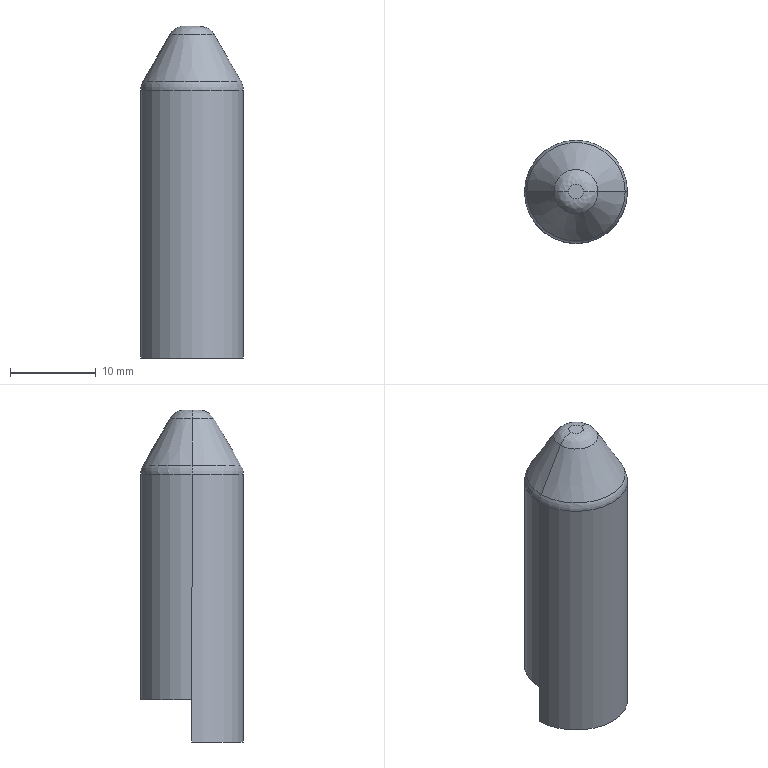Part | STEP file | 1 solid | 16 faces | box 12 x 12 x 38.7 mm | volume 3601 mm3 | plane 6 | cylinder 4 | other 2 | torus 2 | cone 2 | commonest cylinder face diameters 12 x2 5.2 x1 7.4 x1
STEP:
#1=CARTESIAN_POINT('',(0.,0.,0.));
#2=DIRECTION('',(0.,0.,1.));
#3=DIRECTION('',(1.,0.,0.));
#4=AXIS2_PLACEMENT_3D('',#1,#2,#3);
#5=CARTESIAN_POINT('',(6.,0.,-3.7));
#6=VERTEX_POINT('',#5);
#7=CARTESIAN_POINT('',(2.6,0.,-3.7));
#8=VERTEX_POINT('',#7);
#9=CARTESIAN_POINT('',(7.5,0.,-3.7));
#10=DIRECTION('',(-1.,0.,0.));
#11=VECTOR('',#10,1.);
#12=LINE('',#9,#11);
#13=CARTESIAN_POINT('',(7.5,0.,18.));
#14=DIRECTION('',(0.,-1.,0.));
#15=DIRECTION('',(-1.,0.,0.));
#16=AXIS2_PLACEMENT_3D('',#13,#14,#15);
#17=PLANE('',#16);
#18=CARTESIAN_POINT('',(0.,21.7));
#19=DIRECTION('',(1.,0.));
#20=VECTOR('',#19,1.);
#21=LINE('',#18,#20);
#22=(GEOMETRIC_REPRESENTATION_CONTEXT(2)PARAMETRIC_REPRESENTATION_CONTEXT()REPRESENTATION_CONTEXT('',''));
#23=DEFINITIONAL_REPRESENTATION('',(#21),#22);
#24=PCURVE('',#17,#23);
#25=CARTESIAN_POINT('',(0.,0.,-3.7));
#26=DIRECTION('',(0.,0.,1.));
#27=DIRECTION('',(1.,0.,0.));
#28=AXIS2_PLACEMENT_3D('',#25,#26,#27);
#29=PLANE('',#28);
#30=CARTESIAN_POINT('',(7.5,0.));
#31=DIRECTION('',(-1.,0.));
#32=VECTOR('',#31,1.);
#33=LINE('',#30,#32);
#34=(GEOMETRIC_REPRESENTATION_CONTEXT(2)PARAMETRIC_REPRESENTATION_CONTEXT()REPRESENTATION_CONTEXT('',''));
#35=DEFINITIONAL_REPRESENTATION('',(#33),#34);
#36=PCURVE('',#29,#35);
#37=SURFACE_CURVE('',#12,(#24,#36),.PCURVE_S1.);
#38=EDGE_CURVE('',#6,#8,#37,.T.);
#39=ORIENTED_EDGE('',*,*,#38,.T.);
#40=CARTESIAN_POINT('',(2.6,0.,-2.2));
#41=VERTEX_POINT('',#40);
#42=CARTESIAN_POINT('',(2.6,0.,-11.));
#43=DIRECTION('',(0.,0.,-1.));
#44=VECTOR('',#43,1.);
#45=LINE('',#42,#44);
#46=CARTESIAN_POINT('',(4.9,29.));
#47=DIRECTION('',(0.,1.));
#48=VECTOR('',#47,1.);
#49=LINE('',#46,#48);
#50=(GEOMETRIC_REPRESENTATION_CONTEXT(2)PARAMETRIC_REPRESENTATION_CONTEXT()REPRESENTATION_CONTEXT('',''));
#51=DEFINITIONAL_REPRESENTATION('',(#49),#50);
#52=PCURVE('',#17,#51);
#53=CARTESIAN_POINT('',(0.,0.,-11.));
#54=DIRECTION('',(0.,0.,-1.));
#55=DIRECTION('',(0.,1.,0.));
#56=AXIS2_PLACEMENT_3D('',#53,#54,#55);
#57=CYLINDRICAL_SURFACE('',#56,2.6);
#58=CARTESIAN_POINT('',(1.571,0.));
#59=DIRECTION('',(0.,1.));
#60=VECTOR('',#59,1.);
#61=LINE('',#58,#60);
#62=(GEOMETRIC_REPRESENTATION_CONTEXT(2)PARAMETRIC_REPRESENTATION_CONTEXT()REPRESENTATION_CONTEXT('',''));
#63=DEFINITIONAL_REPRESENTATION('',(#61),#62);
#64=PCURVE('',#57,#63);
#65=SURFACE_CURVE('',#45,(#52,#64),.PCURVE_S1.);
#66=EDGE_CURVE('',#41,#8,#65,.T.);
#67=ORIENTED_EDGE('',*,*,#66,.F.);
#68=CARTESIAN_POINT('',(3.7,0.,-2.2));
#69=VERTEX_POINT('',#68);
#70=CARTESIAN_POINT('',(0.,0.,-2.2));
#71=DIRECTION('',(-1.,0.,0.));
#72=VECTOR('',#71,1.);
#73=LINE('',#70,#72);
#74=CARTESIAN_POINT('',(7.5,20.2));
#75=DIRECTION('',(1.,0.));
#76=VECTOR('',#75,1.);
#77=LINE('',#74,#76);
#78=(GEOMETRIC_REPRESENTATION_CONTEXT(2)PARAMETRIC_REPRESENTATION_CONTEXT()REPRESENTATION_CONTEXT('',''));
#79=DEFINITIONAL_REPRESENTATION('',(#77),#78);
#80=PCURVE('',#17,#79);
#81=CARTESIAN_POINT('',(0.,3.7,-2.2));
#82=DIRECTION('',(0.,0.,-1.));
#83=DIRECTION('',(-1.,0.,0.));
#84=AXIS2_PLACEMENT_3D('',#81,#82,#83);
#85=PLANE('',#84);
#86=CARTESIAN_POINT('',(0.,-3.7));
#87=DIRECTION('',(1.,0.));
#88=VECTOR('',#87,1.);
#89=LINE('',#86,#88);
#90=(GEOMETRIC_REPRESENTATION_CONTEXT(2)PARAMETRIC_REPRESENTATION_CONTEXT()REPRESENTATION_CONTEXT('',''));
#91=DEFINITIONAL_REPRESENTATION('',(#89),#90);
#92=PCURVE('',#85,#91);
#93=SURFACE_CURVE('',#73,(#80,#92),.PCURVE_S1.);
#94=EDGE_CURVE('',#69,#41,#93,.T.);
#95=ORIENTED_EDGE('',*,*,#94,.F.);
#96=CARTESIAN_POINT('',(3.7,0.,1.2));
#97=VERTEX_POINT('',#96);
#98=CARTESIAN_POINT('',(3.7,0.,-11.));
#99=DIRECTION('',(0.,0.,-1.));
#100=VECTOR('',#99,1.);
#101=LINE('',#98,#100);
#102=CARTESIAN_POINT('',(3.8,29.));
#103=DIRECTION('',(0.,1.));
#104=VECTOR('',#103,1.);
#105=LINE('',#102,#104);
#106=(GEOMETRIC_REPRESENTATION_CONTEXT(2)PARAMETRIC_REPRESENTATION_CONTEXT()REPRESENTATION_CONTEXT('',''));
#107=DEFINITIONAL_REPRESENTATION('',(#105),#106);
#108=PCURVE('',#17,#107);
#109=CARTESIAN_POINT('',(0.,0.,-11.));
#110=DIRECTION('',(0.,0.,-1.));
#111=DIRECTION('',(0.,1.,0.));
#112=AXIS2_PLACEMENT_3D('',#109,#110,#111);
#113=CYLINDRICAL_SURFACE('',#112,3.7);
#114=CARTESIAN_POINT('',(1.571,0.));
#115=DIRECTION('',(0.,1.));
#116=VECTOR('',#115,1.);
#117=LINE('',#114,#116);
#118=(GEOMETRIC_REPRESENTATION_CONTEXT(2)PARAMETRIC_REPRESENTATION_CONTEXT()REPRESENTATION_CONTEXT('',''));
#119=DEFINITIONAL_REPRESENTATION('',(#117),#118);
#120=PCURVE('',#113,#119);
#121=SURFACE_CURVE('',#101,(#108,#120),.PCURVE_S1.);
#122=EDGE_CURVE('',#97,#69,#121,.T.);
#123=ORIENTED_EDGE('',*,*,#122,.F.);
#124=CARTESIAN_POINT('',(6.,0.,1.2));
#125=VERTEX_POINT('',#124);
#126=CARTESIAN_POINT('',(7.5,0.,1.2));
#127=DIRECTION('',(-1.,0.,0.));
#128=VECTOR('',#127,1.);
#129=LINE('',#126,#128);
#130=CARTESIAN_POINT('',(0.,16.8));
#131=DIRECTION('',(1.,0.));
#132=VECTOR('',#131,1.);
#133=LINE('',#130,#132);
#134=(GEOMETRIC_REPRESENTATION_CONTEXT(2)PARAMETRIC_REPRESENTATION_CONTEXT()REPRESENTATION_CONTEXT('',''));
#135=DEFINITIONAL_REPRESENTATION('',(#133),#134);
#136=PCURVE('',#17,#135);
#137=CARTESIAN_POINT('',(0.,0.,1.2));
#138=DIRECTION('',(0.,0.,1.));
#139=DIRECTION('',(0.,-1.,0.));
#140=AXIS2_PLACEMENT_3D('',#137,#138,#139);
#141=PLANE('',#140);
#142=CARTESIAN_POINT('',(0.,7.5));
#143=DIRECTION('',(0.,-1.));
#144=VECTOR('',#143,1.);
#145=LINE('',#142,#144);
#146=(GEOMETRIC_REPRESENTATION_CONTEXT(2)PARAMETRIC_REPRESENTATION_CONTEXT()REPRESENTATION_CONTEXT('',''));
#147=DEFINITIONAL_REPRESENTATION('',(#145),#146);
#148=PCURVE('',#141,#147);
#149=SURFACE_CURVE('',#129,(#136,#148),.PCURVE_S1.);
#150=EDGE_CURVE('',#125,#97,#149,.T.);
#151=ORIENTED_EDGE('',*,*,#150,.F.);
#152=CARTESIAN_POINT('',(6.,0.,35.));
#153=DIRECTION('',(0.,0.,1.));
#154=VECTOR('',#153,1.);
#155=LINE('',#152,#154);
#156=CARTESIAN_POINT('',(1.5,-17.));
#157=DIRECTION('',(0.,-1.));
#158=VECTOR('',#157,1.);
#159=LINE('',#156,#158);
#160=(GEOMETRIC_REPRESENTATION_CONTEXT(2)PARAMETRIC_REPRESENTATION_CONTEXT()REPRESENTATION_CONTEXT('',''));
#161=DEFINITIONAL_REPRESENTATION('',(#159),#160);
#162=PCURVE('',#17,#161);
#163=CARTESIAN_POINT('',(0.,0.,35.));
#164=DIRECTION('',(0.,0.,-1.));
#165=DIRECTION('',(-1.,0.,0.));
#166=AXIS2_PLACEMENT_3D('',#163,#164,#165);
#167=CYLINDRICAL_SURFACE('',#166,6.);
#168=CARTESIAN_POINT('',(3.142,0.));
#169=DIRECTION('',(0.,-1.));
#170=VECTOR('',#169,1.);
#171=LINE('',#168,#170);
#172=(GEOMETRIC_REPRESENTATION_CONTEXT(2)PARAMETRIC_REPRESENTATION_CONTEXT()REPRESENTATION_CONTEXT('',''));
#173=DEFINITIONAL_REPRESENTATION('',(#171),#172);
#174=PCURVE('',#167,#173);
#175=SURFACE_CURVE('',#155,(#162,#174),.PCURVE_S1.);
#176=EDGE_CURVE('',#6,#125,#175,.T.);
#177=ORIENTED_EDGE('',*,*,#176,.F.);
#178=EDGE_LOOP('',(#39,#67,#95,#123,#151,#177));
#179=FACE_BOUND('',#178,.T.);
#180=ADVANCED_FACE('',(#179),#17,.F.);
#181=CARTESIAN_POINT('',(-3.7,0.,1.2));
#182=VERTEX_POINT('',#181);
#183=CARTESIAN_POINT('',(-6.,0.,1.2));
#184=VERTEX_POINT('',#183);
#185=CARTESIAN_POINT('',(7.5,0.,1.2));
#186=DIRECTION('',(-1.,0.,0.));
#187=VECTOR('',#186,1.);
#188=LINE('',#185,#187);
#189=CARTESIAN_POINT('',(7.5,0.,18.));
#190=DIRECTION('',(0.,-1.,0.));
#191=DIRECTION('',(-1.,0.,0.));
#192=AXIS2_PLACEMENT_3D('',#189,#190,#191);
#193=PLANE('',#192);
#194=CARTESIAN_POINT('',(0.,16.8));
#195=DIRECTION('',(1.,0.));
#196=VECTOR('',#195,1.);
#197=LINE('',#194,#196);
#198=(GEOMETRIC_REPRESENTATION_CONTEXT(2)PARAMETRIC_REPRESENTATION_CONTEXT()REPRESENTATION_CONTEXT('',''));
#199=DEFINITIONAL_REPRESENTATION('',(#197),#198);
#200=PCURVE('',#193,#199);
#201=CARTESIAN_POINT('',(0.,7.5));
#202=DIRECTION('',(0.,-1.));
#203=VECTOR('',#202,1.);
#204=LINE('',#201,#203);
#205=(GEOMETRIC_REPRESENTATION_CONTEXT(2)PARAMETRIC_REPRESENTATION_CONTEXT()REPRESENTATION_CONTEXT('',''));
#206=DEFINITIONAL_REPRESENTATION('',(#204),#205);
#207=PCURVE('',#141,#206);
#208=SURFACE_CURVE('',#188,(#200,#207),.PCURVE_S1.);
#209=EDGE_CURVE('',#182,#184,#208,.T.);
#210=ORIENTED_EDGE('',*,*,#209,.F.);
#211=CARTESIAN_POINT('',(-3.7,0.,-2.2));
#212=VERTEX_POINT('',#211);
#213=CARTESIAN_POINT('',(-3.7,0.,-11.));
#214=DIRECTION('',(0.,0.,1.));
#215=VECTOR('',#214,1.);
#216=LINE('',#213,#215);
#217=CARTESIAN_POINT('',(11.2,29.));
#218=DIRECTION('',(0.,-1.));
#219=VECTOR('',#218,1.);
#220=LINE('',#217,#219);
#221=(GEOMETRIC_REPRESENTATION_CONTEXT(2)PARAMETRIC_REPRESENTATION_CONTEXT()REPRESENTATION_CONTEXT('',''));
#222=DEFINITIONAL_REPRESENTATION('',(#220),#221);
#223=PCURVE('',#193,#222);
#224=CARTESIAN_POINT('',(4.712,0.));
#225=DIRECTION('',(0.,-1.));
#226=VECTOR('',#225,1.);
#227=LINE('',#224,#226);
#228=(GEOMETRIC_REPRESENTATION_CONTEXT(2)PARAMETRIC_REPRESENTATION_CONTEXT()REPRESENTATION_CONTEXT('',''));
#229=DEFINITIONAL_REPRESENTATION('',(#227),#228);
#230=PCURVE('',#113,#229);
#231=SURFACE_CURVE('',#216,(#223,#230),.PCURVE_S1.);
#232=EDGE_CURVE('',#212,#182,#231,.T.);
#233=ORIENTED_EDGE('',*,*,#232,.F.);
#234=CARTESIAN_POINT('',(-2.6,0.,-2.2));
#235=VERTEX_POINT('',#234);
#236=CARTESIAN_POINT('',(0.,0.,-2.2));
#237=DIRECTION('',(-1.,0.,0.));
#238=VECTOR('',#237,1.);
#239=LINE('',#236,#238);
#240=CARTESIAN_POINT('',(7.5,20.2));
#241=DIRECTION('',(1.,0.));
#242=VECTOR('',#241,1.);
#243=LINE('',#240,#242);
#244=(GEOMETRIC_REPRESENTATION_CONTEXT(2)PARAMETRIC_REPRESENTATION_CONTEXT()REPRESENTATION_CONTEXT('',''));
#245=DEFINITIONAL_REPRESENTATION('',(#243),#244);
#246=PCURVE('',#193,#245);
#247=CARTESIAN_POINT('',(0.,-3.7));
#248=DIRECTION('',(1.,0.));
#249=VECTOR('',#248,1.);
#250=LINE('',#247,#249);
#251=(GEOMETRIC_REPRESENTATION_CONTEXT(2)PARAMETRIC_REPRESENTATION_CONTEXT()REPRESENTATION_CONTEXT('',''));
#252=DEFINITIONAL_REPRESENTATION('',(#250),#251);
#253=PCURVE('',#85,#252);
#254=SURFACE_CURVE('',#239,(#246,#253),.PCURVE_S1.);
#255=EDGE_CURVE('',#235,#212,#254,.T.);
#256=ORIENTED_EDGE('',*,*,#255,.F.);
#257=CARTESIAN_POINT('',(-2.6,0.,-3.7));
#258=VERTEX_POINT('',#257);
#259=CARTESIAN_POINT('',(-2.6,0.,-3.7));
#260=DIRECTION('',(0.,0.,1.));
#261=VECTOR('',#260,1.);
#262=LINE('',#259,#261);
#263=CARTESIAN_POINT('',(10.1,21.7));
#264=DIRECTION('',(0.,-1.));
#265=VECTOR('',#264,1.);
#266=LINE('',#263,#265);
#267=(GEOMETRIC_REPRESENTATION_CONTEXT(2)PARAMETRIC_REPRESENTATION_CONTEXT()REPRESENTATION_CONTEXT('',''));
#268=DEFINITIONAL_REPRESENTATION('',(#266),#267);
#269=PCURVE('',#193,#268);
#270=CARTESIAN_POINT('',(4.712,-7.3));
#271=DIRECTION('',(0.,-1.));
#272=VECTOR('',#271,1.);
#273=LINE('',#270,#272);
#274=(GEOMETRIC_REPRESENTATION_CONTEXT(2)PARAMETRIC_REPRESENTATION_CONTEXT()REPRESENTATION_CONTEXT('',''));
#275=DEFINITIONAL_REPRESENTATION('',(#273),#274);
#276=PCURVE('',#57,#275);
#277=SURFACE_CURVE('',#262,(#269,#276),.PCURVE_S1.);
#278=EDGE_CURVE('',#258,#235,#277,.T.);
#279=ORIENTED_EDGE('',*,*,#278,.F.);
#280=CARTESIAN_POINT('',(-6.,0.,-3.7));
#281=VERTEX_POINT('',#280);
#282=CARTESIAN_POINT('',(7.5,0.,-3.7));
#283=DIRECTION('',(-1.,0.,0.));
#284=VECTOR('',#283,1.);
#285=LINE('',#282,#284);
#286=CARTESIAN_POINT('',(0.,21.7));
#287=DIRECTION('',(1.,0.));
#288=VECTOR('',#287,1.);
#289=LINE('',#286,#288);
#290=(GEOMETRIC_REPRESENTATION_CONTEXT(2)PARAMETRIC_REPRESENTATION_CONTEXT()REPRESENTATION_CONTEXT('',''));
#291=DEFINITIONAL_REPRESENTATION('',(#289),#290);
#292=PCURVE('',#193,#291);
#293=CARTESIAN_POINT('',(7.5,0.));
#294=DIRECTION('',(-1.,0.));
#295=VECTOR('',#294,1.);
#296=LINE('',#293,#295);
#297=(GEOMETRIC_REPRESENTATION_CONTEXT(2)PARAMETRIC_REPRESENTATION_CONTEXT()REPRESENTATION_CONTEXT('',''));
#298=DEFINITIONAL_REPRESENTATION('',(#296),#297);
#299=PCURVE('',#29,#298);
#300=SURFACE_CURVE('',#285,(#292,#299),.PCURVE_S1.);
#301=EDGE_CURVE('',#258,#281,#300,.T.);
#302=ORIENTED_EDGE('',*,*,#301,.T.);
#303=CARTESIAN_POINT('',(-6.,0.,35.));
#304=DIRECTION('',(0.,0.,-1.));
#305=VECTOR('',#304,1.);
#306=LINE('',#303,#305);
#307=CARTESIAN_POINT('',(13.5,-17.));
#308=DIRECTION('',(0.,1.));
#309=VECTOR('',#308,1.);
#310=LINE('',#307,#309);
#311=(GEOMETRIC_REPRESENTATION_CONTEXT(2)PARAMETRIC_REPRESENTATION_CONTEXT()REPRESENTATION_CONTEXT('',''));
#312=DEFINITIONAL_REPRESENTATION('',(#310),#311);
#313=PCURVE('',#193,#312);
#314=CARTESIAN_POINT('',(6.283,0.));
#315=DIRECTION('',(0.,1.));
#316=VECTOR('',#315,1.);
#317=LINE('',#314,#316);
#318=(GEOMETRIC_REPRESENTATION_CONTEXT(2)PARAMETRIC_REPRESENTATION_CONTEXT()REPRESENTATION_CONTEXT('',''));
#319=DEFINITIONAL_REPRESENTATION('',(#317),#318);
#320=PCURVE('',#167,#319);
#321=SURFACE_CURVE('',#306,(#313,#320),.PCURVE_S1.);
#322=EDGE_CURVE('',#184,#281,#321,.T.);
#323=ORIENTED_EDGE('',*,*,#322,.F.);
#324=EDGE_LOOP('',(#210,#233,#256,#279,#302,#323));
#325=FACE_BOUND('',#324,.T.);
#326=ADVANCED_FACE('',(#325),#193,.F.);
#327=CARTESIAN_POINT('',(0.,0.,-2.2));
#328=DIRECTION('',(0.,0.,-1.));
#329=DIRECTION('',(0.,1.,0.));
#330=AXIS2_PLACEMENT_3D('',#327,#328,#329);
#331=CIRCLE('',#330,3.7);
#332=CARTESIAN_POINT('',(0.,-3.7));
#333=DIRECTION('',(0.,1.));
#334=AXIS2_PLACEMENT_2D('',#332,#333);
#335=CIRCLE('',#334,3.7);
#336=(GEOMETRIC_REPRESENTATION_CONTEXT(2)PARAMETRIC_REPRESENTATION_CONTEXT()REPRESENTATION_CONTEXT('',''));
#337=DEFINITIONAL_REPRESENTATION('',(#335),#336);
#338=PCURVE('',#85,#337);
#339=CARTESIAN_POINT('',(0.,-8.8));
#340=DIRECTION('',(1.,0.));
#341=VECTOR('',#340,1.);
#342=LINE('',#339,#341);
#343=(GEOMETRIC_REPRESENTATION_CONTEXT(2)PARAMETRIC_REPRESENTATION_CONTEXT()REPRESENTATION_CONTEXT('',''));
#344=DEFINITIONAL_REPRESENTATION('',(#342),#343);
#345=PCURVE('',#113,#344);
#346=SURFACE_CURVE('',#331,(#338,#345),.PCURVE_S1.);
#347=EDGE_CURVE('',#69,#212,#346,.T.);
#348=ORIENTED_EDGE('',*,*,#347,.F.);
#349=ORIENTED_EDGE('',*,*,#94,.T.);
#350=CARTESIAN_POINT('',(0.,0.,-2.2));
#351=DIRECTION('',(0.,0.,-1.));
#352=DIRECTION('',(0.,1.,0.));
#353=AXIS2_PLACEMENT_3D('',#350,#351,#352);
#354=CIRCLE('',#353,2.6);
#355=CARTESIAN_POINT('',(0.,-3.7));
#356=DIRECTION('',(0.,1.));
#357=AXIS2_PLACEMENT_2D('',#355,#356);
#358=CIRCLE('',#357,2.6);
#359=(GEOMETRIC_REPRESENTATION_CONTEXT(2)PARAMETRIC_REPRESENTATION_CONTEXT()REPRESENTATION_CONTEXT('',''));
#360=DEFINITIONAL_REPRESENTATION('',(#358),#359);
#361=PCURVE('',#85,#360);
#362=CARTESIAN_POINT('',(0.,-8.8));
#363=DIRECTION('',(1.,0.));
#364=VECTOR('',#363,1.);
#365=LINE('',#362,#364);
#366=(GEOMETRIC_REPRESENTATION_CONTEXT(2)PARAMETRIC_REPRESENTATION_CONTEXT()REPRESENTATION_CONTEXT('',''));
#367=DEFINITIONAL_REPRESENTATION('',(#365),#366);
#368=PCURVE('',#57,#367);
#369=SURFACE_CURVE('',#354,(#361,#368),.PCURVE_S1.);
#370=EDGE_CURVE('',#41,#235,#369,.T.);
#371=ORIENTED_EDGE('',*,*,#370,.T.);
#372=ORIENTED_EDGE('',*,*,#255,.T.);
#373=EDGE_LOOP('',(#348,#349,#371,#372));
#374=FACE_BOUND('',#373,.T.);
#375=ADVANCED_FACE('',(#374),#85,.F.);
#376=ORIENTED_EDGE('',*,*,#122,.F.);
#377=CARTESIAN_POINT('',(0.,0.,1.2));
#378=DIRECTION('',(0.,0.,-1.));
#379=DIRECTION('',(0.,-1.,0.));
#380=AXIS2_PLACEMENT_3D('',#377,#378,#379);
#381=CIRCLE('',#380,3.7);
#382=CARTESIAN_POINT('',(-3.142,-12.2));
#383=DIRECTION('',(1.,0.));
#384=VECTOR('',#383,1.);
#385=LINE('',#382,#384);
#386=(GEOMETRIC_REPRESENTATION_CONTEXT(2)PARAMETRIC_REPRESENTATION_CONTEXT()REPRESENTATION_CONTEXT('',''));
#387=DEFINITIONAL_REPRESENTATION('',(#385),#386);
#388=PCURVE('',#113,#387);
#389=CARTESIAN_POINT('',(3.7,0.));
#390=CARTESIAN_POINT('',(3.7,-6.409));
#391=CARTESIAN_POINT('',(-1.85,-3.204));
#392=CARTESIAN_POINT('',(-7.4,0.));
#393=CARTESIAN_POINT('',(-1.85,3.204));
#394=CARTESIAN_POINT('',(3.7,6.409));
#395=CARTESIAN_POINT('',(3.7,0.));
#396=(BOUNDED_CURVE()B_SPLINE_CURVE(2,(#389,#390,#391,#392,#393,#394,#395),.UNSPECIFIED.,.T.,.F.)B_SPLINE_CURVE_WITH_KNOTS((1,2,2,2,2,1),(-2.094,0.,2.094,4.189,6.283,8.378),.UNSPECIFIED.)CURVE()GEOMETRIC_REPRESENTATION_ITEM()RATIONAL_B_SPLINE_CURVE((1.,0.5,1.,0.5,1.,0.5,1.))REPRESENTATION_ITEM(''));
#397=(GEOMETRIC_REPRESENTATION_CONTEXT(2)PARAMETRIC_REPRESENTATION_CONTEXT()REPRESENTATION_CONTEXT('',''));
#398=DEFINITIONAL_REPRESENTATION('',(#396),#397);
#399=PCURVE('',#141,#398);
#400=SURFACE_CURVE('',#381,(#388,#399),.PCURVE_S1.);
#401=EDGE_CURVE('',#97,#182,#400,.T.);
#402=ORIENTED_EDGE('',*,*,#401,.T.);
#403=ORIENTED_EDGE('',*,*,#232,.F.);
#404=ORIENTED_EDGE('',*,*,#347,.F.);
#405=EDGE_LOOP('',(#376,#402,#403,#404));
#406=FACE_BOUND('',#405,.F.);
#407=ADVANCED_FACE('',(#406),#113,.F.);
#408=ORIENTED_EDGE('',*,*,#401,.T.);
#409=ORIENTED_EDGE('',*,*,#209,.T.);
#410=CARTESIAN_POINT('',(0.,0.,1.2));
#411=DIRECTION('',(0.,0.,1.));
#412=DIRECTION('',(0.,-1.,0.));
#413=AXIS2_PLACEMENT_3D('',#410,#411,#412);
#414=CIRCLE('',#413,6.);
#415=CARTESIAN_POINT('',(0.,0.));
#416=DIRECTION('',(1.,0.));
#417=AXIS2_PLACEMENT_2D('',#415,#416);
#418=CIRCLE('',#417,6.);
#419=(GEOMETRIC_REPRESENTATION_CONTEXT(2)PARAMETRIC_REPRESENTATION_CONTEXT()REPRESENTATION_CONTEXT('',''));
#420=DEFINITIONAL_REPRESENTATION('',(#418),#419);
#421=PCURVE('',#141,#420);
#422=CARTESIAN_POINT('',(0.,0.,35.));
#423=DIRECTION('',(0.,0.,-1.));
#424=DIRECTION('',(-1.,0.,0.));
#425=AXIS2_PLACEMENT_3D('',#422,#423,#424);
#426=CYLINDRICAL_SURFACE('',#425,6.);
#427=CARTESIAN_POINT('',(4.712,33.8));
#428=DIRECTION('',(-1.,0.));
#429=VECTOR('',#428,1.);
#430=LINE('',#427,#429);
#431=(GEOMETRIC_REPRESENTATION_CONTEXT(2)PARAMETRIC_REPRESENTATION_CONTEXT()REPRESENTATION_CONTEXT('',''));
#432=DEFINITIONAL_REPRESENTATION('',(#430),#431);
#433=PCURVE('',#426,#432);
#434=SURFACE_CURVE('',#414,(#421,#433),.PCURVE_S1.);
#435=EDGE_CURVE('',#125,#184,#434,.T.);
#436=ORIENTED_EDGE('',*,*,#435,.F.);
#437=ORIENTED_EDGE('',*,*,#150,.T.);
#438=EDGE_LOOP('',(#408,#409,#436,#437));
#439=FACE_BOUND('',#438,.T.);
#440=ADVANCED_FACE('',(#439),#141,.F.);
#441=ORIENTED_EDGE('',*,*,#66,.F.);
#442=ORIENTED_EDGE('',*,*,#370,.T.);
#443=ORIENTED_EDGE('',*,*,#278,.F.);
#444=CARTESIAN_POINT('',(0.,0.,-3.7));
#445=DIRECTION('',(0.,0.,1.));
#446=DIRECTION('',(1.,0.,0.));
#447=AXIS2_PLACEMENT_3D('',#444,#445,#446);
#448=CIRCLE('',#447,2.6);
#449=CARTESIAN_POINT('',(7.854,-7.3));
#450=DIRECTION('',(-1.,0.));
#451=VECTOR('',#450,1.);
#452=LINE('',#449,#451);
#453=(GEOMETRIC_REPRESENTATION_CONTEXT(2)PARAMETRIC_REPRESENTATION_CONTEXT()REPRESENTATION_CONTEXT('',''));
#454=DEFINITIONAL_REPRESENTATION('',(#452),#453);
#455=PCURVE('',#57,#454);
#456=CARTESIAN_POINT('',(0.,0.));
#457=DIRECTION('',(1.,0.));
#458=AXIS2_PLACEMENT_2D('',#456,#457);
#459=CIRCLE('',#458,2.6);
#460=(GEOMETRIC_REPRESENTATION_CONTEXT(2)PARAMETRIC_REPRESENTATION_CONTEXT()REPRESENTATION_CONTEXT('',''));
#461=DEFINITIONAL_REPRESENTATION('',(#459),#460);
#462=PCURVE('',#29,#461);
#463=SURFACE_CURVE('',#448,(#455,#462),.PCURVE_S1.);
#464=EDGE_CURVE('',#258,#8,#463,.T.);
#465=ORIENTED_EDGE('',*,*,#464,.T.);
#466=EDGE_LOOP('',(#441,#442,#443,#465));
#467=FACE_BOUND('',#466,.F.);
#468=ADVANCED_FACE('',(#467),#57,.F.);
#469=CARTESIAN_POINT('',(-2.577,0.,34.));
#470=VERTEX_POINT('',#469);
#471=CARTESIAN_POINT('',(-0.8453,0.,35.));
#472=VERTEX_POINT('',#471);
#473=CARTESIAN_POINT('',(-0.8453,0.,33.));
#474=DIRECTION('',(0.,1.,0.));
#475=DIRECTION('',(-1.,0.,0.));
#476=AXIS2_PLACEMENT_3D('',#473,#474,#475);
#477=CIRCLE('',#476,2.);
#478=CARTESIAN_POINT('',(2.577,0.,34.));
#479=CARTESIAN_POINT('',(2.403,0.,34.302));
#480=CARTESIAN_POINT('',(2.165,0.,34.568));
#481=CARTESIAN_POINT('',(1.873,0.,34.781));
#482=CARTESIAN_POINT('',(1.543,0.,34.927));
#483=CARTESIAN_POINT('',(1.194,0.,35.));
#484=CARTESIAN_POINT('',(0.8453,0.,35.));
#485=B_SPLINE_CURVE_WITH_KNOTS('',6,(#478,#479,#480,#481,#482,#483,#484),.UNSPECIFIED.,.F.,.F.,(7,7),(0.5236,1.571),.PIECEWISE_BEZIER_KNOTS.);
#486=CARTESIAN_POINT('',(0.,0.,33.));
#487=DIRECTION('',(0.,0.,1.));
#488=AXIS1_PLACEMENT('',#486,#487);
#489=SURFACE_OF_REVOLUTION('',#485,#488);
#490=CARTESIAN_POINT('',(3.142,0.));
#491=DIRECTION('',(0.,1.));
#492=VECTOR('',#491,1.);
#493=LINE('',#490,#492);
#494=(GEOMETRIC_REPRESENTATION_CONTEXT(2)PARAMETRIC_REPRESENTATION_CONTEXT()REPRESENTATION_CONTEXT('',''));
#495=DEFINITIONAL_REPRESENTATION('',(#493),#494);
#496=PCURVE('',#489,#495);
#497=CARTESIAN_POINT('',(2.577,0.,34.));
#498=CARTESIAN_POINT('',(2.403,0.,34.302));
#499=CARTESIAN_POINT('',(2.165,0.,34.568));
#500=CARTESIAN_POINT('',(1.873,0.,34.781));
#501=CARTESIAN_POINT('',(1.543,0.,34.927));
#502=CARTESIAN_POINT('',(1.194,0.,35.));
#503=CARTESIAN_POINT('',(0.8453,0.,35.));
#504=B_SPLINE_CURVE_WITH_KNOTS('',6,(#497,#498,#499,#500,#501,#502,#503),.UNSPECIFIED.,.F.,.F.,(7,7),(0.5236,1.571),.PIECEWISE_BEZIER_KNOTS.);
#505=CARTESIAN_POINT('',(0.,0.,33.));
#506=DIRECTION('',(0.,0.,1.));
#507=AXIS1_PLACEMENT('',#505,#506);
#508=SURFACE_OF_REVOLUTION('',#504,#507);
#509=CARTESIAN_POINT('',(3.142,0.));
#510=DIRECTION('',(0.,1.));
#511=VECTOR('',#510,1.);
#512=LINE('',#509,#511);
#513=(GEOMETRIC_REPRESENTATION_CONTEXT(2)PARAMETRIC_REPRESENTATION_CONTEXT()REPRESENTATION_CONTEXT('',''));
#514=DEFINITIONAL_REPRESENTATION('',(#512),#513);
#515=PCURVE('',#508,#514);
#516=SURFACE_CURVE('',#477,(#496,#515),.PCURVE_S1.);
#517=EDGE_CURVE('',#470,#472,#516,.T.);
#518=ORIENTED_EDGE('',*,*,#517,.F.);
#519=CARTESIAN_POINT('',(2.577,0.,34.));
#520=VERTEX_POINT('',#519);
#521=CARTESIAN_POINT('',(0.,0.,34.));
#522=DIRECTION('',(0.,0.,-1.));
#523=DIRECTION('',(1.,0.,0.));
#524=AXIS2_PLACEMENT_3D('',#521,#522,#523);
#525=CIRCLE('',#524,2.577);
#526=CARTESIAN_POINT('',(6.283,0.5236));
#527=DIRECTION('',(-1.,0.));
#528=VECTOR('',#527,1.);
#529=LINE('',#526,#528);
#530=(GEOMETRIC_REPRESENTATION_CONTEXT(2)PARAMETRIC_REPRESENTATION_CONTEXT()REPRESENTATION_CONTEXT('',''));
#531=DEFINITIONAL_REPRESENTATION('',(#529),#530);
#532=PCURVE('',#489,#531);
#533=CARTESIAN_POINT('',(0.,0.,35.));
#534=DIRECTION('',(0.,0.,-1.));
#535=DIRECTION('',(-1.,0.,0.));
#536=AXIS2_PLACEMENT_3D('',#533,#534,#535);
#537=CONICAL_SURFACE('',#536,2.,0.5236);
#538=CARTESIAN_POINT('',(3.142,1.));
#539=DIRECTION('',(1.,0.));
#540=VECTOR('',#539,1.);
#541=LINE('',#538,#540);
#542=(GEOMETRIC_REPRESENTATION_CONTEXT(2)PARAMETRIC_REPRESENTATION_CONTEXT()REPRESENTATION_CONTEXT('',''));
#543=DEFINITIONAL_REPRESENTATION('',(#541),#542);
#544=PCURVE('',#537,#543);
#545=SURFACE_CURVE('',#525,(#532,#544),.PCURVE_S1.);
#546=EDGE_CURVE('',#520,#470,#545,.T.);
#547=ORIENTED_EDGE('',*,*,#546,.F.);
#548=CARTESIAN_POINT('',(0.8453,0.,35.));
#549=VERTEX_POINT('',#548);
#550=CARTESIAN_POINT('',(0.8453,0.,33.));
#551=DIRECTION('',(0.,-1.,0.));
#552=DIRECTION('',(0.,0.,-1.));
#553=AXIS2_PLACEMENT_3D('',#550,#551,#552);
#554=CIRCLE('',#553,2.);
#555=CARTESIAN_POINT('',(6.283,-1.571));
#556=DIRECTION('',(0.,1.));
#557=VECTOR('',#556,1.);
#558=LINE('',#555,#557);
#559=(GEOMETRIC_REPRESENTATION_CONTEXT(2)PARAMETRIC_REPRESENTATION_CONTEXT()REPRESENTATION_CONTEXT('',''));
#560=DEFINITIONAL_REPRESENTATION('',(#558),#559);
#561=PCURVE('',#489,#560);
#562=CARTESIAN_POINT('',(0.,-1.571));
#563=DIRECTION('',(0.,1.));
#564=VECTOR('',#563,1.);
#565=LINE('',#562,#564);
#566=(GEOMETRIC_REPRESENTATION_CONTEXT(2)PARAMETRIC_REPRESENTATION_CONTEXT()REPRESENTATION_CONTEXT('',''));
#567=DEFINITIONAL_REPRESENTATION('',(#565),#566);
#568=PCURVE('',#508,#567);
#569=SURFACE_CURVE('',#554,(#561,#568),.PCURVE_S1.);
#570=EDGE_CURVE('',#520,#549,#569,.T.);
#571=ORIENTED_EDGE('',*,*,#570,.T.);
#572=CARTESIAN_POINT('',(0.,0.,35.));
#573=DIRECTION('',(0.,0.,1.));
#574=DIRECTION('',(1.,0.,0.));
#575=AXIS2_PLACEMENT_3D('',#572,#573,#574);
#576=CIRCLE('',#575,0.8453);
#577=CARTESIAN_POINT('',(0.,1.571));
#578=DIRECTION('',(1.,0.));
#579=VECTOR('',#578,1.);
#580=LINE('',#577,#579);
#581=(GEOMETRIC_REPRESENTATION_CONTEXT(2)PARAMETRIC_REPRESENTATION_CONTEXT()REPRESENTATION_CONTEXT('',''));
#582=DEFINITIONAL_REPRESENTATION('',(#580),#581);
#583=PCURVE('',#489,#582);
#584=CARTESIAN_POINT('',(0.,0.,35.));
#585=DIRECTION('',(0.,0.,1.));
#586=DIRECTION('',(1.,0.,0.));
#587=AXIS2_PLACEMENT_3D('',#584,#585,#586);
#588=PLANE('',#587);
#589=CARTESIAN_POINT('',(0.,0.));
#590=DIRECTION('',(1.,0.));
#591=AXIS2_PLACEMENT_2D('',#589,#590);
#592=CIRCLE('',#591,0.8453);
#593=(GEOMETRIC_REPRESENTATION_CONTEXT(2)PARAMETRIC_REPRESENTATION_CONTEXT()REPRESENTATION_CONTEXT('',''));
#594=DEFINITIONAL_REPRESENTATION('',(#592),#593);
#595=PCURVE('',#588,#594);
#596=SURFACE_CURVE('',#576,(#583,#595),.PCURVE_S1.);
#597=EDGE_CURVE('',#472,#549,#596,.T.);
#598=ORIENTED_EDGE('',*,*,#597,.F.);
#599=EDGE_LOOP('',(#518,#547,#571,#598));
#600=FACE_BOUND('',#599,.T.);
#601=ADVANCED_FACE('',(#600),#489,.T.);
#602=CARTESIAN_POINT('',(-6.,0.,27.536));
#603=VERTEX_POINT('',#602);
#604=CARTESIAN_POINT('',(-5.732,0.,28.536));
#605=VERTEX_POINT('',#604);
#606=CARTESIAN_POINT('',(-4.,0.,27.536));
#607=DIRECTION('',(0.,1.,0.));
#608=DIRECTION('',(-1.,0.,0.));
#609=AXIS2_PLACEMENT_3D('',#606,#607,#608);
#610=CIRCLE('',#609,2.);
#611=CARTESIAN_POINT('',(0.,0.,27.536));
#612=DIRECTION('',(0.,0.,1.));
#613=DIRECTION('',(1.,0.,0.));
#614=AXIS2_PLACEMENT_3D('',#611,#612,#613);
#615=TOROIDAL_SURFACE('',#614,4.,2.);
#616=CARTESIAN_POINT('',(3.142,0.));
#617=DIRECTION('',(0.,1.));
#618=VECTOR('',#617,1.);
#619=LINE('',#616,#618);
#620=(GEOMETRIC_REPRESENTATION_CONTEXT(2)PARAMETRIC_REPRESENTATION_CONTEXT()REPRESENTATION_CONTEXT('',''));
#621=DEFINITIONAL_REPRESENTATION('',(#619),#620);
#622=PCURVE('',#615,#621);
#623=CARTESIAN_POINT('',(0.,0.,27.536));
#624=DIRECTION('',(0.,0.,1.));
#625=DIRECTION('',(1.,0.,0.));
#626=AXIS2_PLACEMENT_3D('',#623,#624,#625);
#627=TOROIDAL_SURFACE('',#626,4.,2.);
#628=CARTESIAN_POINT('',(3.142,0.));
#629=DIRECTION('',(0.,1.));
#630=VECTOR('',#629,1.);
#631=LINE('',#628,#630);
#632=(GEOMETRIC_REPRESENTATION_CONTEXT(2)PARAMETRIC_REPRESENTATION_CONTEXT()REPRESENTATION_CONTEXT('',''));
#633=DEFINITIONAL_REPRESENTATION('',(#631),#632);
#634=PCURVE('',#627,#633);
#635=SURFACE_CURVE('',#610,(#622,#634),.PCURVE_S1.);
#636=EDGE_CURVE('',#603,#605,#635,.T.);
#637=ORIENTED_EDGE('',*,*,#636,.F.);
#638=CARTESIAN_POINT('',(6.,0.,27.536));
#639=VERTEX_POINT('',#638);
#640=CARTESIAN_POINT('',(0.,0.,27.536));
#641=DIRECTION('',(0.,0.,-1.));
#642=DIRECTION('',(1.,0.,0.));
#643=AXIS2_PLACEMENT_3D('',#640,#641,#642);
#644=CIRCLE('',#643,6.);
#645=CARTESIAN_POINT('',(6.283,0.));
#646=DIRECTION('',(-1.,0.));
#647=VECTOR('',#646,1.);
#648=LINE('',#645,#647);
#649=(GEOMETRIC_REPRESENTATION_CONTEXT(2)PARAMETRIC_REPRESENTATION_CONTEXT()REPRESENTATION_CONTEXT('',''));
#650=DEFINITIONAL_REPRESENTATION('',(#648),#649);
#651=PCURVE('',#615,#650);
#652=CARTESIAN_POINT('',(3.142,7.464));
#653=DIRECTION('',(1.,0.));
#654=VECTOR('',#653,1.);
#655=LINE('',#652,#654);
#656=(GEOMETRIC_REPRESENTATION_CONTEXT(2)PARAMETRIC_REPRESENTATION_CONTEXT()REPRESENTATION_CONTEXT('',''));
#657=DEFINITIONAL_REPRESENTATION('',(#655),#656);
#658=PCURVE('',#167,#657);
#659=SURFACE_CURVE('',#644,(#651,#658),.PCURVE_S1.);
#660=EDGE_CURVE('',#639,#603,#659,.T.);
#661=ORIENTED_EDGE('',*,*,#660,.F.);
#662=CARTESIAN_POINT('',(5.732,0.,28.536));
#663=VERTEX_POINT('',#662);
#664=CARTESIAN_POINT('',(4.,0.,27.536));
#665=DIRECTION('',(0.,-1.,0.));
#666=DIRECTION('',(0.,0.,-1.));
#667=AXIS2_PLACEMENT_3D('',#664,#665,#666);
#668=CIRCLE('',#667,2.);
#669=CARTESIAN_POINT('',(6.283,-1.571));
#670=DIRECTION('',(0.,1.));
#671=VECTOR('',#670,1.);
#672=LINE('',#669,#671);
#673=(GEOMETRIC_REPRESENTATION_CONTEXT(2)PARAMETRIC_REPRESENTATION_CONTEXT()REPRESENTATION_CONTEXT('',''));
#674=DEFINITIONAL_REPRESENTATION('',(#672),#673);
#675=PCURVE('',#615,#674);
#676=CARTESIAN_POINT('',(0.,-1.571));
#677=DIRECTION('',(0.,1.));
#678=VECTOR('',#677,1.);
#679=LINE('',#676,#678);
#680=(GEOMETRIC_REPRESENTATION_CONTEXT(2)PARAMETRIC_REPRESENTATION_CONTEXT()REPRESENTATION_CONTEXT('',''));
#681=DEFINITIONAL_REPRESENTATION('',(#679),#680);
#682=PCURVE('',#627,#681);
#683=SURFACE_CURVE('',#668,(#675,#682),.PCURVE_S1.);
#684=EDGE_CURVE('',#639,#663,#683,.T.);
#685=ORIENTED_EDGE('',*,*,#684,.T.);
#686=CARTESIAN_POINT('',(0.,0.,28.536));
#687=DIRECTION('',(0.,0.,1.));
#688=DIRECTION('',(-1.,0.,0.));
#689=AXIS2_PLACEMENT_3D('',#686,#687,#688);
#690=CIRCLE('',#689,5.732);
#691=CARTESIAN_POINT('',(3.142,0.5236));
#692=DIRECTION('',(1.,0.));
#693=VECTOR('',#692,1.);
#694=LINE('',#691,#693);
#695=(GEOMETRIC_REPRESENTATION_CONTEXT(2)PARAMETRIC_REPRESENTATION_CONTEXT()REPRESENTATION_CONTEXT('',''));
#696=DEFINITIONAL_REPRESENTATION('',(#694),#695);
#697=PCURVE('',#615,#696);
#698=CARTESIAN_POINT('',(6.283,6.464));
#699=DIRECTION('',(-1.,0.));
#700=VECTOR('',#699,1.);
#701=LINE('',#698,#700);
#702=(GEOMETRIC_REPRESENTATION_CONTEXT(2)PARAMETRIC_REPRESENTATION_CONTEXT()REPRESENTATION_CONTEXT('',''));
#703=DEFINITIONAL_REPRESENTATION('',(#701),#702);
#704=PCURVE('',#537,#703);
#705=SURFACE_CURVE('',#690,(#697,#704),.PCURVE_S1.);
#706=EDGE_CURVE('',#605,#663,#705,.T.);
#707=ORIENTED_EDGE('',*,*,#706,.F.);
#708=EDGE_LOOP('',(#637,#661,#685,#707));
#709=FACE_BOUND('',#708,.T.);
#710=ADVANCED_FACE('',(#709),#615,.T.);
#711=CARTESIAN_POINT('',(2.,0.,35.));
#712=DIRECTION('',(0.5,0.,-0.866));
#713=VECTOR('',#712,1.);
#714=LINE('',#711,#713);
#715=CARTESIAN_POINT('',(3.142,0.));
#716=DIRECTION('',(0.,1.));
#717=VECTOR('',#716,1.);
#718=LINE('',#715,#717);
#719=(GEOMETRIC_REPRESENTATION_CONTEXT(2)PARAMETRIC_REPRESENTATION_CONTEXT()REPRESENTATION_CONTEXT('',''));
#720=DEFINITIONAL_REPRESENTATION('',(#718),#719);
#721=PCURVE('',#537,#720);
#722=CARTESIAN_POINT('',(0.,0.,35.));
#723=DIRECTION('',(0.,0.,-1.));
#724=DIRECTION('',(-1.,0.,0.));
#725=AXIS2_PLACEMENT_3D('',#722,#723,#724);
#726=CONICAL_SURFACE('',#725,2.,0.5236);
#727=CARTESIAN_POINT('',(3.142,0.));
#728=DIRECTION('',(0.,1.));
#729=VECTOR('',#728,1.);
#730=LINE('',#727,#729);
#731=(GEOMETRIC_REPRESENTATION_CONTEXT(2)PARAMETRIC_REPRESENTATION_CONTEXT()REPRESENTATION_CONTEXT('',''));
#732=DEFINITIONAL_REPRESENTATION('',(#730),#731);
#733=PCURVE('',#726,#732);
#734=SURFACE_CURVE('',#714,(#721,#733),.PCURVE_S1.);
#735=EDGE_CURVE('',#520,#663,#734,.T.);
#736=ORIENTED_EDGE('',*,*,#735,.F.);
#737=ORIENTED_EDGE('',*,*,#546,.T.);
#738=CARTESIAN_POINT('',(-2.,0.,35.));
#739=DIRECTION('',(-0.5,0.,-0.866));
#740=VECTOR('',#739,1.);
#741=LINE('',#738,#740);
#742=CARTESIAN_POINT('',(6.283,0.));
#743=DIRECTION('',(0.,1.));
#744=VECTOR('',#743,1.);
#745=LINE('',#742,#744);
#746=(GEOMETRIC_REPRESENTATION_CONTEXT(2)PARAMETRIC_REPRESENTATION_CONTEXT()REPRESENTATION_CONTEXT('',''));
#747=DEFINITIONAL_REPRESENTATION('',(#745),#746);
#748=PCURVE('',#537,#747);
#749=CARTESIAN_POINT('',(0.,0.));
#750=DIRECTION('',(0.,1.));
#751=VECTOR('',#750,1.);
#752=LINE('',#749,#751);
#753=(GEOMETRIC_REPRESENTATION_CONTEXT(2)PARAMETRIC_REPRESENTATION_CONTEXT()REPRESENTATION_CONTEXT('',''));
#754=DEFINITIONAL_REPRESENTATION('',(#752),#753);
#755=PCURVE('',#726,#754);
#756=SURFACE_CURVE('',#741,(#748,#755),.PCURVE_S1.);
#757=EDGE_CURVE('',#470,#605,#756,.T.);
#758=ORIENTED_EDGE('',*,*,#757,.T.);
#759=ORIENTED_EDGE('',*,*,#706,.T.);
#760=EDGE_LOOP('',(#736,#737,#758,#759));
#761=FACE_BOUND('',#760,.T.);
#762=ADVANCED_FACE('',(#761),#537,.T.);
#763=CARTESIAN_POINT('',(0.,0.,-3.7));
#764=DIRECTION('',(0.,0.,1.));
#765=DIRECTION('',(1.,0.,0.));
#766=AXIS2_PLACEMENT_3D('',#763,#764,#765);
#767=CIRCLE('',#766,6.);
#768=CARTESIAN_POINT('',(0.,0.));
#769=DIRECTION('',(1.,0.));
#770=AXIS2_PLACEMENT_2D('',#768,#769);
#771=CIRCLE('',#770,6.);
#772=(GEOMETRIC_REPRESENTATION_CONTEXT(2)PARAMETRIC_REPRESENTATION_CONTEXT()REPRESENTATION_CONTEXT('',''));
#773=DEFINITIONAL_REPRESENTATION('',(#771),#772);
#774=PCURVE('',#29,#773);
#775=CARTESIAN_POINT('',(9.425,38.7));
#776=DIRECTION('',(-1.,0.));
#777=VECTOR('',#776,1.);
#778=LINE('',#775,#777);
#779=(GEOMETRIC_REPRESENTATION_CONTEXT(2)PARAMETRIC_REPRESENTATION_CONTEXT()REPRESENTATION_CONTEXT('',''));
#780=DEFINITIONAL_REPRESENTATION('',(#778),#779);
#781=PCURVE('',#167,#780);
#782=SURFACE_CURVE('',#767,(#774,#781),.PCURVE_S1.);
#783=EDGE_CURVE('',#281,#6,#782,.T.);
#784=ORIENTED_EDGE('',*,*,#783,.F.);
#785=ORIENTED_EDGE('',*,*,#301,.F.);
#786=ORIENTED_EDGE('',*,*,#464,.T.);
#787=ORIENTED_EDGE('',*,*,#38,.F.);
#788=EDGE_LOOP('',(#784,#785,#786,#787));
#789=FACE_BOUND('',#788,.T.);
#790=ADVANCED_FACE('',(#789),#29,.F.);
#791=CARTESIAN_POINT('',(0.,0.,35.));
#792=DIRECTION('',(0.,0.,1.));
#793=DIRECTION('',(1.,0.,0.));
#794=AXIS2_PLACEMENT_3D('',#791,#792,#793);
#795=CIRCLE('',#794,0.8453);
#796=CARTESIAN_POINT('',(0.,0.));
#797=DIRECTION('',(1.,0.));
#798=AXIS2_PLACEMENT_2D('',#796,#797);
#799=CIRCLE('',#798,0.8453);
#800=(GEOMETRIC_REPRESENTATION_CONTEXT(2)PARAMETRIC_REPRESENTATION_CONTEXT()REPRESENTATION_CONTEXT('',''));
#801=DEFINITIONAL_REPRESENTATION('',(#799),#800);
#802=PCURVE('',#588,#801);
#803=CARTESIAN_POINT('',(0.,1.571));
#804=DIRECTION('',(1.,0.));
#805=VECTOR('',#804,1.);
#806=LINE('',#803,#805);
#807=(GEOMETRIC_REPRESENTATION_CONTEXT(2)PARAMETRIC_REPRESENTATION_CONTEXT()REPRESENTATION_CONTEXT('',''));
#808=DEFINITIONAL_REPRESENTATION('',(#806),#807);
#809=PCURVE('',#508,#808);
#810=SURFACE_CURVE('',#795,(#802,#809),.PCURVE_S1.);
#811=EDGE_CURVE('',#549,#472,#810,.T.);
#812=ORIENTED_EDGE('',*,*,#811,.T.);
#813=ORIENTED_EDGE('',*,*,#597,.T.);
#814=EDGE_LOOP('',(#812,#813));
#815=FACE_BOUND('',#814,.T.);
#816=ADVANCED_FACE('',(#815),#588,.T.);
#817=CARTESIAN_POINT('',(6.,0.,35.));
#818=DIRECTION('',(0.,0.,-1.));
#819=VECTOR('',#818,1.);
#820=LINE('',#817,#819);
#821=CARTESIAN_POINT('',(3.142,0.));
#822=DIRECTION('',(0.,1.));
#823=VECTOR('',#822,1.);
#824=LINE('',#821,#823);
#825=(GEOMETRIC_REPRESENTATION_CONTEXT(2)PARAMETRIC_REPRESENTATION_CONTEXT()REPRESENTATION_CONTEXT('',''));
#826=DEFINITIONAL_REPRESENTATION('',(#824),#825);
#827=PCURVE('',#167,#826);
#828=CARTESIAN_POINT('',(3.142,0.));
#829=DIRECTION('',(0.,1.));
#830=VECTOR('',#829,1.);
#831=LINE('',#828,#830);
#832=(GEOMETRIC_REPRESENTATION_CONTEXT(2)PARAMETRIC_REPRESENTATION_CONTEXT()REPRESENTATION_CONTEXT('',''));
#833=DEFINITIONAL_REPRESENTATION('',(#831),#832);
#834=PCURVE('',#426,#833);
#835=SURFACE_CURVE('',#820,(#827,#834),.PCURVE_S1.);
#836=EDGE_CURVE('',#639,#125,#835,.T.);
#837=ORIENTED_EDGE('',*,*,#836,.F.);
#838=ORIENTED_EDGE('',*,*,#660,.T.);
#839=CARTESIAN_POINT('',(-6.,0.,35.));
#840=DIRECTION('',(0.,0.,-1.));
#841=VECTOR('',#840,1.);
#842=LINE('',#839,#841);
#843=CARTESIAN_POINT('',(6.283,0.));
#844=DIRECTION('',(0.,1.));
#845=VECTOR('',#844,1.);
#846=LINE('',#843,#845);
#847=(GEOMETRIC_REPRESENTATION_CONTEXT(2)PARAMETRIC_REPRESENTATION_CONTEXT()REPRESENTATION_CONTEXT('',''));
#848=DEFINITIONAL_REPRESENTATION('',(#846),#847);
#849=PCURVE('',#167,#848);
#850=CARTESIAN_POINT('',(0.,0.));
#851=DIRECTION('',(0.,1.));
#852=VECTOR('',#851,1.);
#853=LINE('',#850,#852);
#854=(GEOMETRIC_REPRESENTATION_CONTEXT(2)PARAMETRIC_REPRESENTATION_CONTEXT()REPRESENTATION_CONTEXT('',''));
#855=DEFINITIONAL_REPRESENTATION('',(#853),#854);
#856=PCURVE('',#426,#855);
#857=SURFACE_CURVE('',#842,(#849,#856),.PCURVE_S1.);
#858=EDGE_CURVE('',#603,#184,#857,.T.);
#859=ORIENTED_EDGE('',*,*,#858,.T.);
#860=ORIENTED_EDGE('',*,*,#322,.T.);
#861=ORIENTED_EDGE('',*,*,#783,.T.);
#862=ORIENTED_EDGE('',*,*,#176,.T.);
#863=EDGE_LOOP('',(#837,#838,#859,#860,#861,#862));
#864=FACE_BOUND('',#863,.T.);
#865=ADVANCED_FACE('',(#864),#167,.T.);
#866=CARTESIAN_POINT('',(0.,0.,27.536));
#867=DIRECTION('',(0.,0.,-1.));
#868=DIRECTION('',(1.,0.,0.));
#869=AXIS2_PLACEMENT_3D('',#866,#867,#868);
#870=CIRCLE('',#869,6.);
#871=CARTESIAN_POINT('',(-3.142,7.464));
#872=DIRECTION('',(1.,0.));
#873=VECTOR('',#872,1.);
#874=LINE('',#871,#873);
#875=(GEOMETRIC_REPRESENTATION_CONTEXT(2)PARAMETRIC_REPRESENTATION_CONTEXT()REPRESENTATION_CONTEXT('',''));
#876=DEFINITIONAL_REPRESENTATION('',(#874),#875);
#877=PCURVE('',#426,#876);
#878=CARTESIAN_POINT('',(6.283,0.));
#879=DIRECTION('',(-1.,0.));
#880=VECTOR('',#879,1.);
#881=LINE('',#878,#880);
#882=(GEOMETRIC_REPRESENTATION_CONTEXT(2)PARAMETRIC_REPRESENTATION_CONTEXT()REPRESENTATION_CONTEXT('',''));
#883=DEFINITIONAL_REPRESENTATION('',(#881),#882);
#884=PCURVE('',#627,#883);
#885=SURFACE_CURVE('',#870,(#877,#884),.PCURVE_S1.);
#886=EDGE_CURVE('',#603,#639,#885,.T.);
#887=ORIENTED_EDGE('',*,*,#886,.T.);
#888=ORIENTED_EDGE('',*,*,#836,.T.);
#889=ORIENTED_EDGE('',*,*,#435,.T.);
#890=ORIENTED_EDGE('',*,*,#858,.F.);
#891=EDGE_LOOP('',(#887,#888,#889,#890));
#892=FACE_BOUND('',#891,.T.);
#893=ADVANCED_FACE('',(#892),#426,.T.);
#894=CARTESIAN_POINT('',(0.,0.,34.));
#895=DIRECTION('',(0.,0.,-1.));
#896=DIRECTION('',(1.,0.,0.));
#897=AXIS2_PLACEMENT_3D('',#894,#895,#896);
#898=CIRCLE('',#897,2.577);
#899=CARTESIAN_POINT('',(-3.142,1.));
#900=DIRECTION('',(1.,0.));
#901=VECTOR('',#900,1.);
#902=LINE('',#899,#901);
#903=(GEOMETRIC_REPRESENTATION_CONTEXT(2)PARAMETRIC_REPRESENTATION_CONTEXT()REPRESENTATION_CONTEXT('',''));
#904=DEFINITIONAL_REPRESENTATION('',(#902),#903);
#905=PCURVE('',#726,#904);
#906=CARTESIAN_POINT('',(6.283,0.5236));
#907=DIRECTION('',(-1.,0.));
#908=VECTOR('',#907,1.);
#909=LINE('',#906,#908);
#910=(GEOMETRIC_REPRESENTATION_CONTEXT(2)PARAMETRIC_REPRESENTATION_CONTEXT()REPRESENTATION_CONTEXT('',''));
#911=DEFINITIONAL_REPRESENTATION('',(#909),#910);
#912=PCURVE('',#508,#911);
#913=SURFACE_CURVE('',#898,(#905,#912),.PCURVE_S1.);
#914=EDGE_CURVE('',#470,#520,#913,.T.);
#915=ORIENTED_EDGE('',*,*,#914,.T.);
#916=ORIENTED_EDGE('',*,*,#735,.T.);
#917=CARTESIAN_POINT('',(0.,0.,28.536));
#918=DIRECTION('',(0.,0.,1.));
#919=DIRECTION('',(-1.,0.,0.));
#920=AXIS2_PLACEMENT_3D('',#917,#918,#919);
#921=CIRCLE('',#920,5.732);
#922=CARTESIAN_POINT('',(6.283,6.464));
#923=DIRECTION('',(-1.,0.));
#924=VECTOR('',#923,1.);
#925=LINE('',#922,#924);
#926=(GEOMETRIC_REPRESENTATION_CONTEXT(2)PARAMETRIC_REPRESENTATION_CONTEXT()REPRESENTATION_CONTEXT('',''));
#927=DEFINITIONAL_REPRESENTATION('',(#925),#926);
#928=PCURVE('',#726,#927);
#929=CARTESIAN_POINT('',(-3.142,0.5236));
#930=DIRECTION('',(1.,0.));
#931=VECTOR('',#930,1.);
#932=LINE('',#929,#931);
#933=(GEOMETRIC_REPRESENTATION_CONTEXT(2)PARAMETRIC_REPRESENTATION_CONTEXT()REPRESENTATION_CONTEXT('',''));
#934=DEFINITIONAL_REPRESENTATION('',(#932),#933);
#935=PCURVE('',#627,#934);
#936=SURFACE_CURVE('',#921,(#928,#935),.PCURVE_S1.);
#937=EDGE_CURVE('',#663,#605,#936,.T.);
#938=ORIENTED_EDGE('',*,*,#937,.T.);
#939=ORIENTED_EDGE('',*,*,#757,.F.);
#940=EDGE_LOOP('',(#915,#916,#938,#939));
#941=FACE_BOUND('',#940,.T.);
#942=ADVANCED_FACE('',(#941),#726,.T.);
#943=ORIENTED_EDGE('',*,*,#886,.F.);
#944=ORIENTED_EDGE('',*,*,#636,.T.);
#945=ORIENTED_EDGE('',*,*,#937,.F.);
#946=ORIENTED_EDGE('',*,*,#684,.F.);
#947=EDGE_LOOP('',(#943,#944,#945,#946));
#948=FACE_BOUND('',#947,.T.);
#949=ADVANCED_FACE('',(#948),#627,.T.);
#950=ORIENTED_EDGE('',*,*,#914,.F.);
#951=ORIENTED_EDGE('',*,*,#517,.T.);
#952=ORIENTED_EDGE('',*,*,#811,.F.);
#953=ORIENTED_EDGE('',*,*,#570,.F.);
#954=EDGE_LOOP('',(#950,#951,#952,#953));
#955=FACE_BOUND('',#954,.T.);
#956=ADVANCED_FACE('',(#955),#508,.T.);
#957=CLOSED_SHELL('',(#180,#326,#375,#407,#440,#468,#601,#710,#762,#790,#816,#865,#893,#942,#949,#956));
#958=MANIFOLD_SOLID_BREP('',#957);
#959=(LENGTH_UNIT()NAMED_UNIT(*)SI_UNIT(.MILLI.,.METRE.));
#960=UNCERTAINTY_MEASURE_WITH_UNIT(LENGTH_MEASURE(0.0000001),#959,'','');
#961=(NAMED_UNIT(*)PLANE_ANGLE_UNIT()SI_UNIT($,.RADIAN.));
#962=(NAMED_UNIT(*)SI_UNIT($,.STERADIAN.)SOLID_ANGLE_UNIT());
#963=(GEOMETRIC_REPRESENTATION_CONTEXT(3)GLOBAL_UNCERTAINTY_ASSIGNED_CONTEXT((#960))GLOBAL_UNIT_ASSIGNED_CONTEXT((#959,#961,#962))REPRESENTATION_CONTEXT('',''));
#964=ADVANCED_BREP_SHAPE_REPRESENTATION('',(#4,#958),#963);